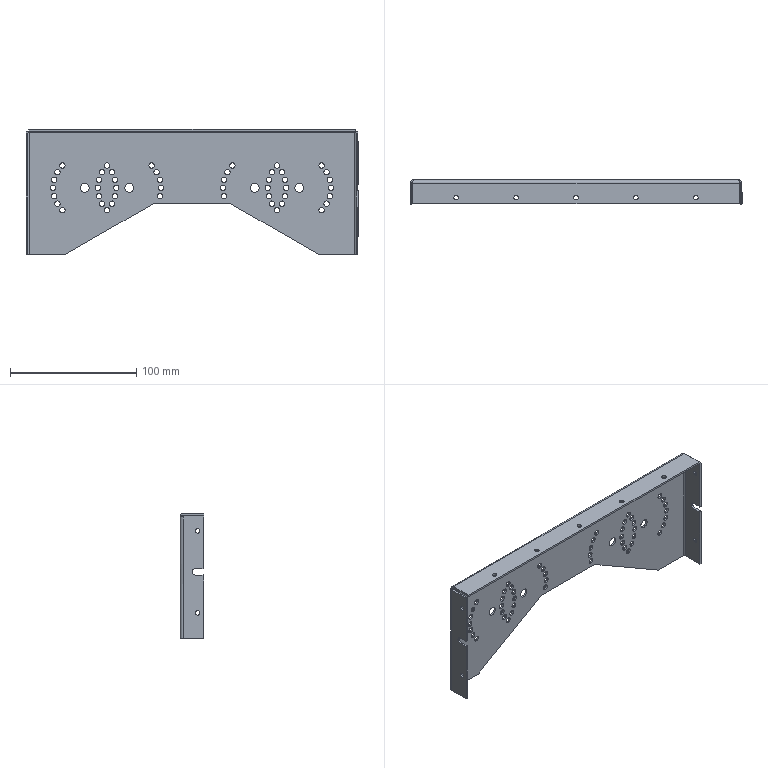Part | SolidWorks | features HoleWzd 6, Fillet 4, Cut 3, EdgeFlange 2, MirrorPattern 2, FlatPattern 1, ICE 1, SMBaseFlange 1, SheetMetal 1 | 1 solid | 170 faces | box 263 x 19 x 99.5 mm | volume 41053 mm3 | cylinder 136 | plane 30 | spline 4 | commonest cylinder face diameters 4.3 x96 3.6 x18 5 x11 7 x8 2 x3